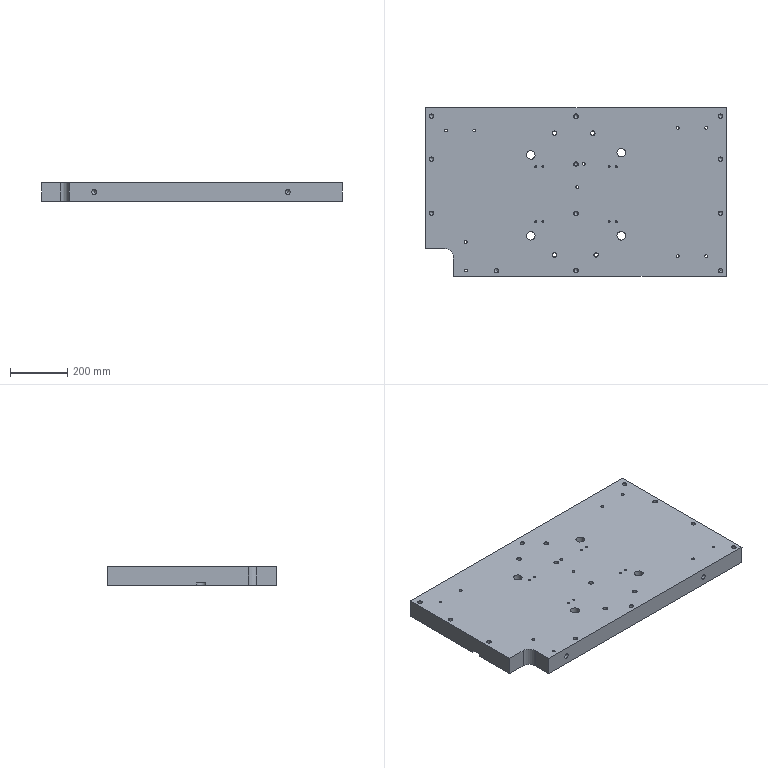Part | NX | features solid 2 | 1 solid | 363 faces | box 1050 x 590 x 65 mm | volume 37627031 mm3 | cone 180 | cylinder 141 | plane 42 | commonest cylinder face diameters 14 x36 8.5 x20 6.8 x16 10.3 x16 10 x10 7 x8